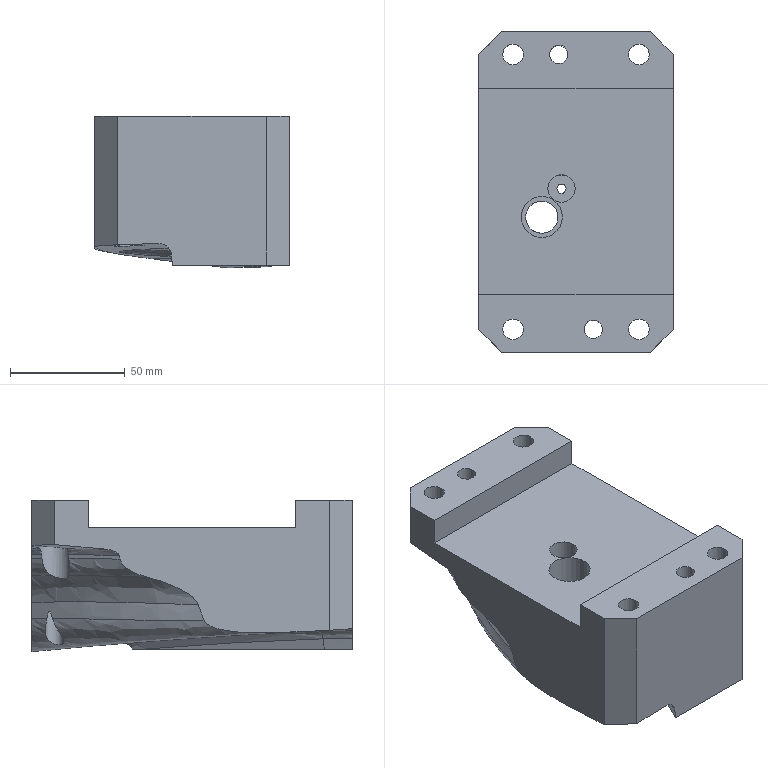Part | NX | features solid 2 | 1 solid | 63 faces | box 85.003 x 140.002 x 66.255 mm | volume 538477 mm3 | spline 29 | plane 20 | cylinder 14 | commonest cylinder face diameters 9 x4 14 x4 8 x2 4 x1 12 x1 14.1 x1